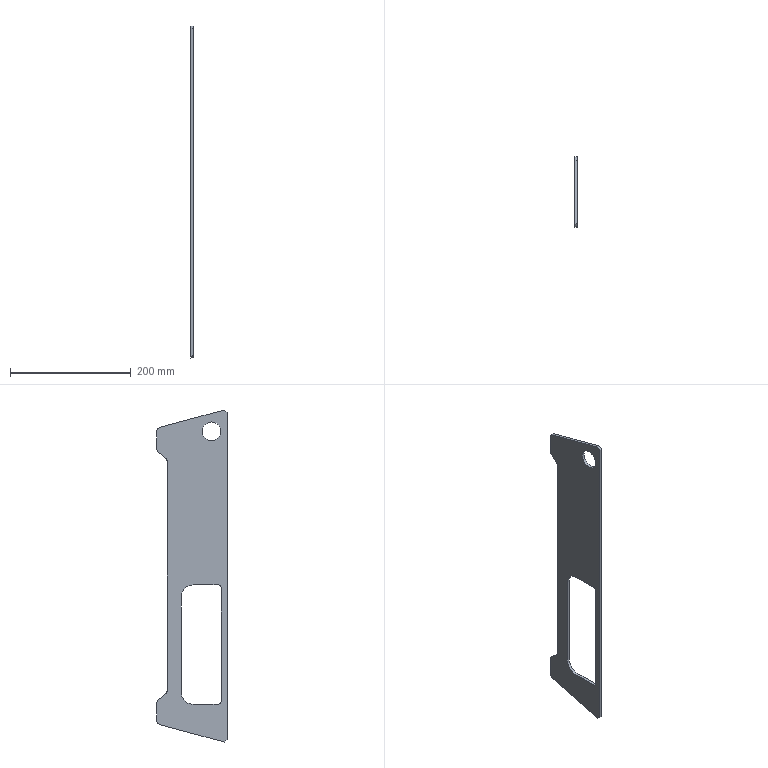Part | SolidWorks | features BaseBody 1 | 1 solid | 28 faces | box 4.5 x 116.8 x 550.797 mm | volume 181763 mm3 | plane 16 | cylinder 12 | commonest cylinder face diameters 16 x4 10 x2 12 x2 31 x2 40 x2
STEP:
#1=CARTESIAN_POINT('',(1093.2,55.3,688.5));
#2=VERTEX_POINT('',#1);
#3=CARTESIAN_POINT('',(1093.2,55.3,719.5));
#4=VERTEX_POINT('',#3);
#5=CARTESIAN_POINT('',(1093.2,55.3,704.));
#6=DIRECTION('',(-1.,0.,0.));
#7=DIRECTION('',(0.,0.,-1.));
#8=AXIS2_PLACEMENT_3D('',#5,#6,#7);
#9=CIRCLE('',#8,15.5);
#10=EDGE_CURVE('',#2,#4,#9,.T.);
#11=ORIENTED_EDGE('',*,*,#10,.T.);
#12=CARTESIAN_POINT('',(1097.7,55.3,719.5));
#13=VERTEX_POINT('',#12);
#14=CARTESIAN_POINT('',(1093.2,55.3,719.5));
#15=DIRECTION('',(1.,0.,0.));
#16=VECTOR('',#15,1000.);
#17=LINE('',#14,#16);
#18=EDGE_CURVE('',#4,#13,#17,.T.);
#19=ORIENTED_EDGE('',*,*,#18,.T.);
#20=CARTESIAN_POINT('',(1097.7,55.3,688.5));
#21=VERTEX_POINT('',#20);
#22=CARTESIAN_POINT('',(1097.7,55.3,704.));
#23=DIRECTION('',(-1.,0.,0.));
#24=DIRECTION('',(0.,0.,-1.));
#25=AXIS2_PLACEMENT_3D('',#22,#23,#24);
#26=CIRCLE('',#25,15.5);
#27=EDGE_CURVE('',#21,#13,#26,.T.);
#28=ORIENTED_EDGE('',*,*,#27,.F.);
#29=CARTESIAN_POINT('',(1093.2,55.3,688.5));
#30=DIRECTION('',(1.,0.,0.));
#31=VECTOR('',#30,1000.);
#32=LINE('',#29,#31);
#33=EDGE_CURVE('',#2,#21,#32,.T.);
#34=ORIENTED_EDGE('',*,*,#33,.F.);
#35=EDGE_LOOP('',(#11,#19,#28,#34));
#36=FACE_OUTER_BOUND('',#35,.T.);
#37=CARTESIAN_POINT('',(1093.2,55.3,704.));
#38=DIRECTION('',(1.,0.,0.));
#39=DIRECTION('',(0.,0.,-1.));
#40=AXIS2_PLACEMENT_3D('',#37,#38,#39);
#41=CYLINDRICAL_SURFACE('',#40,15.5);
#42=ADVANCED_FACE('',(#36),#41,.F.);
#43=CARTESIAN_POINT('',(1097.7,39.3,444.2));
#44=VERTEX_POINT('',#43);
#45=CARTESIAN_POINT('',(1097.7,44.3,449.2));
#46=VERTEX_POINT('',#45);
#47=CARTESIAN_POINT('',(1097.7,44.3,444.2));
#48=DIRECTION('',(-1.,0.,0.));
#49=DIRECTION('',(0.,0.,1.));
#50=AXIS2_PLACEMENT_3D('',#47,#48,#49);
#51=CIRCLE('',#50,5.);
#52=EDGE_CURVE('',#44,#46,#51,.T.);
#53=ORIENTED_EDGE('',*,*,#52,.T.);
#54=CARTESIAN_POINT('',(1097.7,85.7,449.2));
#55=VERTEX_POINT('',#54);
#56=CARTESIAN_POINT('',(1097.7,87.7,449.2));
#57=DIRECTION('',(0.,1.,0.));
#58=VECTOR('',#57,1000.);
#59=LINE('',#56,#58);
#60=EDGE_CURVE('',#46,#55,#59,.T.);
#61=ORIENTED_EDGE('',*,*,#60,.T.);
#62=CARTESIAN_POINT('',(1097.7,105.7,429.2));
#63=VERTEX_POINT('',#62);
#64=CARTESIAN_POINT('',(1097.7,85.7,429.2));
#65=DIRECTION('',(-1.,0.,0.));
#66=DIRECTION('',(0.,0.,1.));
#67=AXIS2_PLACEMENT_3D('',#64,#65,#66);
#68=CIRCLE('',#67,20.);
#69=EDGE_CURVE('',#55,#63,#68,.T.);
#70=ORIENTED_EDGE('',*,*,#69,.T.);
#71=CARTESIAN_POINT('',(1097.7,105.7,271.2));
#72=VERTEX_POINT('',#71);
#73=CARTESIAN_POINT('',(1097.7,105.7,464.));
#74=DIRECTION('',(0.,0.,-1.));
#75=VECTOR('',#74,1000.);
#76=LINE('',#73,#75);
#77=EDGE_CURVE('',#63,#72,#76,.T.);
#78=ORIENTED_EDGE('',*,*,#77,.T.);
#79=CARTESIAN_POINT('',(1097.7,85.7,251.2));
#80=VERTEX_POINT('',#79);
#81=CARTESIAN_POINT('',(1097.7,85.7,271.2));
#82=DIRECTION('',(-1.,0.,0.));
#83=DIRECTION('',(0.,0.,1.));
#84=AXIS2_PLACEMENT_3D('',#81,#82,#83);
#85=CIRCLE('',#84,20.);
#86=EDGE_CURVE('',#72,#80,#85,.T.);
#87=ORIENTED_EDGE('',*,*,#86,.T.);
#88=CARTESIAN_POINT('',(1097.7,44.3,251.2));
#89=VERTEX_POINT('',#88);
#90=CARTESIAN_POINT('',(1097.7,87.7,251.2));
#91=DIRECTION('',(0.,-1.,0.));
#92=VECTOR('',#91,1000.);
#93=LINE('',#90,#92);
#94=EDGE_CURVE('',#80,#89,#93,.T.);
#95=ORIENTED_EDGE('',*,*,#94,.T.);
#96=CARTESIAN_POINT('',(1097.7,39.3,256.2));
#97=VERTEX_POINT('',#96);
#98=CARTESIAN_POINT('',(1097.7,44.3,256.2));
#99=DIRECTION('',(-1.,0.,0.));
#100=DIRECTION('',(0.,0.,1.));
#101=AXIS2_PLACEMENT_3D('',#98,#99,#100);
#102=CIRCLE('',#101,5.);
#103=EDGE_CURVE('',#89,#97,#102,.T.);
#104=ORIENTED_EDGE('',*,*,#103,.T.);
#105=CARTESIAN_POINT('',(1097.7,39.3,464.));
#106=DIRECTION('',(0.,0.,1.));
#107=VECTOR('',#106,1000.);
#108=LINE('',#105,#107);
#109=EDGE_CURVE('',#97,#44,#108,.T.);
#110=ORIENTED_EDGE('',*,*,#109,.T.);
#111=EDGE_LOOP('',(#53,#61,#70,#78,#87,#95,#104,#110));
#112=FACE_BOUND('',#111,.T.);
#113=ORIENTED_EDGE('',*,*,#27,.T.);
#114=CARTESIAN_POINT('',(1097.7,55.3,704.));
#115=DIRECTION('',(-1.,0.,0.));
#116=DIRECTION('',(0.,0.,-1.));
#117=AXIS2_PLACEMENT_3D('',#114,#115,#116);
#118=CIRCLE('',#117,15.5);
#119=EDGE_CURVE('',#13,#21,#118,.T.);
#120=ORIENTED_EDGE('',*,*,#119,.T.);
#121=EDGE_LOOP('',(#113,#120));
#122=FACE_BOUND('',#121,.T.);
#123=CARTESIAN_POINT('',(1097.7,29.3,735.693));
#124=VERTEX_POINT('',#123);
#125=CARTESIAN_POINT('',(1097.7,29.3,192.307));
#126=VERTEX_POINT('',#125);
#127=CARTESIAN_POINT('',(1097.7,29.3,464.));
#128=DIRECTION('',(0.,0.,-1.));
#129=VECTOR('',#128,1000.);
#130=LINE('',#127,#129);
#131=EDGE_CURVE('',#124,#126,#130,.T.);
#132=ORIENTED_EDGE('',*,*,#131,.T.);
#133=CARTESIAN_POINT('',(1097.7,34.13,188.602));
#134=VERTEX_POINT('',#133);
#135=CARTESIAN_POINT('',(1097.7,29.3,192.307));
#136=DIRECTION('',(0.,0.7934,-0.6088));
#137=VECTOR('',#136,1000.);
#138=LINE('',#135,#137);
#139=EDGE_CURVE('',#126,#134,#138,.T.);
#140=ORIENTED_EDGE('',*,*,#139,.T.);
#141=CARTESIAN_POINT('',(1097.7,140.171,217.015));
#142=VERTEX_POINT('',#141);
#143=CARTESIAN_POINT('',(1097.7,34.13,188.602));
#144=DIRECTION('',(0.,0.9659,0.2588));
#145=VECTOR('',#144,1000.);
#146=LINE('',#143,#145);
#147=EDGE_CURVE('',#134,#142,#146,.T.);
#148=ORIENTED_EDGE('',*,*,#147,.T.);
#149=CARTESIAN_POINT('',(1097.7,146.1,224.743));
#150=VERTEX_POINT('',#149);
#151=CARTESIAN_POINT('',(1097.7,138.1,224.743));
#152=DIRECTION('',(1.,0.,0.));
#153=DIRECTION('',(0.,0.,1.));
#154=AXIS2_PLACEMENT_3D('',#151,#152,#153);
#155=CIRCLE('',#154,8.);
#156=EDGE_CURVE('',#142,#150,#155,.T.);
#157=ORIENTED_EDGE('',*,*,#156,.T.);
#158=CARTESIAN_POINT('',(1097.7,146.1,252.393));
#159=VERTEX_POINT('',#158);
#160=CARTESIAN_POINT('',(1097.7,146.1,464.));
#161=DIRECTION('',(0.,0.,1.));
#162=VECTOR('',#161,1000.);
#163=LINE('',#160,#162);
#164=EDGE_CURVE('',#150,#159,#163,.T.);
#165=ORIENTED_EDGE('',*,*,#164,.T.);
#166=CARTESIAN_POINT('',(1097.7,143.186,258.568));
#167=VERTEX_POINT('',#166);
#168=CARTESIAN_POINT('',(1097.7,138.1,252.393));
#169=DIRECTION('',(1.,0.,0.));
#170=DIRECTION('',(0.,0.,1.));
#171=AXIS2_PLACEMENT_3D('',#168,#169,#170);
#172=CIRCLE('',#171,8.);
#173=EDGE_CURVE('',#159,#167,#172,.T.);
#174=ORIENTED_EDGE('',*,*,#173,.T.);
#175=CARTESIAN_POINT('',(1097.7,131.286,268.368));
#176=VERTEX_POINT('',#175);
#177=CARTESIAN_POINT('',(1097.7,143.186,258.568));
#178=DIRECTION('',(0.,-0.7719,0.6357));
#179=VECTOR('',#178,1000.);
#180=LINE('',#177,#179);
#181=EDGE_CURVE('',#167,#176,#180,.T.);
#182=ORIENTED_EDGE('',*,*,#181,.T.);
#183=CARTESIAN_POINT('',(1097.7,129.1,273.));
#184=VERTEX_POINT('',#183);
#185=CARTESIAN_POINT('',(1097.7,135.1,273.));
#186=DIRECTION('',(-1.,0.,0.));
#187=DIRECTION('',(0.,0.,-1.));
#188=AXIS2_PLACEMENT_3D('',#185,#186,#187);
#189=CIRCLE('',#188,6.);
#190=EDGE_CURVE('',#176,#184,#189,.T.);
#191=ORIENTED_EDGE('',*,*,#190,.T.);
#192=CARTESIAN_POINT('',(1097.7,129.1,655.));
#193=VERTEX_POINT('',#192);
#194=CARTESIAN_POINT('',(1097.7,129.1,464.));
#195=DIRECTION('',(0.,0.,1.));
#196=VECTOR('',#195,1000.);
#197=LINE('',#194,#196);
#198=EDGE_CURVE('',#184,#193,#197,.T.);
#199=ORIENTED_EDGE('',*,*,#198,.T.);
#200=CARTESIAN_POINT('',(1097.7,131.286,659.632));
#201=VERTEX_POINT('',#200);
#202=CARTESIAN_POINT('',(1097.7,135.1,655.));
#203=DIRECTION('',(-1.,0.,0.));
#204=DIRECTION('',(0.,0.,-1.));
#205=AXIS2_PLACEMENT_3D('',#202,#203,#204);
#206=CIRCLE('',#205,6.);
#207=EDGE_CURVE('',#193,#201,#206,.T.);
#208=ORIENTED_EDGE('',*,*,#207,.T.);
#209=CARTESIAN_POINT('',(1097.7,143.186,669.432));
#210=VERTEX_POINT('',#209);
#211=CARTESIAN_POINT('',(1097.7,131.286,659.632));
#212=DIRECTION('',(0.,0.7719,0.6357));
#213=VECTOR('',#212,1000.);
#214=LINE('',#211,#213);
#215=EDGE_CURVE('',#201,#210,#214,.T.);
#216=ORIENTED_EDGE('',*,*,#215,.T.);
#217=CARTESIAN_POINT('',(1097.7,146.1,675.607));
#218=VERTEX_POINT('',#217);
#219=CARTESIAN_POINT('',(1097.7,138.1,675.607));
#220=DIRECTION('',(1.,0.,0.));
#221=DIRECTION('',(0.,0.,1.));
#222=AXIS2_PLACEMENT_3D('',#219,#220,#221);
#223=CIRCLE('',#222,8.);
#224=EDGE_CURVE('',#210,#218,#223,.T.);
#225=ORIENTED_EDGE('',*,*,#224,.T.);
#226=CARTESIAN_POINT('',(1097.7,146.1,703.257));
#227=VERTEX_POINT('',#226);
#228=CARTESIAN_POINT('',(1097.7,146.1,464.));
#229=DIRECTION('',(0.,0.,1.));
#230=VECTOR('',#229,1000.);
#231=LINE('',#228,#230);
#232=EDGE_CURVE('',#218,#227,#231,.T.);
#233=ORIENTED_EDGE('',*,*,#232,.T.);
#234=CARTESIAN_POINT('',(1097.7,140.171,710.985));
#235=VERTEX_POINT('',#234);
#236=CARTESIAN_POINT('',(1097.7,138.1,703.257));
#237=DIRECTION('',(1.,0.,0.));
#238=DIRECTION('',(0.,0.,1.));
#239=AXIS2_PLACEMENT_3D('',#236,#237,#238);
#240=CIRCLE('',#239,8.);
#241=EDGE_CURVE('',#227,#235,#240,.T.);
#242=ORIENTED_EDGE('',*,*,#241,.T.);
#243=CARTESIAN_POINT('',(1097.7,34.13,739.398));
#244=VERTEX_POINT('',#243);
#245=CARTESIAN_POINT('',(1097.7,140.171,710.985));
#246=DIRECTION('',(0.,-0.9659,0.2588));
#247=VECTOR('',#246,1000.);
#248=LINE('',#245,#247);
#249=EDGE_CURVE('',#235,#244,#248,.T.);
#250=ORIENTED_EDGE('',*,*,#249,.T.);
#251=CARTESIAN_POINT('',(1097.7,34.13,739.398));
#252=DIRECTION('',(0.,-0.7934,-0.6088));
#253=VECTOR('',#252,1000.);
#254=LINE('',#251,#253);
#255=EDGE_CURVE('',#244,#124,#254,.T.);
#256=ORIENTED_EDGE('',*,*,#255,.T.);
#257=EDGE_LOOP('',(#132,#140,#148,#157,#165,#174,#182,#191,#199,#208,#216,#225,#233,#242,#250,#256));
#258=FACE_OUTER_BOUND('',#257,.T.);
#259=CARTESIAN_POINT('',(1097.7,29.3,185.297));
#260=DIRECTION('',(1.,0.,0.));
#261=DIRECTION('',(0.,1.,0.));
#262=AXIS2_PLACEMENT_3D('',#259,#260,#261);
#263=PLANE('',#262);
#264=ADVANCED_FACE('',(#112,#122,#258),#263,.T.);
#265=CARTESIAN_POINT('',(1093.2,85.7,449.2));
#266=VERTEX_POINT('',#265);
#267=CARTESIAN_POINT('',(1095.45,85.7,449.2));
#268=DIRECTION('',(-1.,0.,0.));
#269=VECTOR('',#268,1000.);
#270=LINE('',#267,#269);
#271=EDGE_CURVE('',#55,#266,#270,.T.);
#272=ORIENTED_EDGE('',*,*,#271,.F.);
#273=ORIENTED_EDGE('',*,*,#60,.F.);
#274=CARTESIAN_POINT('',(1093.2,44.3,449.2));
#275=VERTEX_POINT('',#274);
#276=CARTESIAN_POINT('',(1095.45,44.3,449.2));
#277=DIRECTION('',(1.,0.,0.));
#278=VECTOR('',#277,1000.);
#279=LINE('',#276,#278);
#280=EDGE_CURVE('',#275,#46,#279,.T.);
#281=ORIENTED_EDGE('',*,*,#280,.F.);
#282=CARTESIAN_POINT('',(1093.2,65.,449.2));
#283=DIRECTION('',(0.,-1.,0.));
#284=VECTOR('',#283,1000.);
#285=LINE('',#282,#284);
#286=EDGE_CURVE('',#266,#275,#285,.T.);
#287=ORIENTED_EDGE('',*,*,#286,.F.);
#288=EDGE_LOOP('',(#272,#273,#281,#287));
#289=FACE_OUTER_BOUND('',#288,.T.);
#290=CARTESIAN_POINT('',(1093.2,44.3,449.2));
#291=DIRECTION('',(0.,0.,1.));
#292=DIRECTION('',(1.,0.,0.));
#293=AXIS2_PLACEMENT_3D('',#290,#291,#292);
#294=PLANE('',#293);
#295=ADVANCED_FACE('',(#289),#294,.F.);
#296=ORIENTED_EDGE('',*,*,#52,.F.);
#297=CARTESIAN_POINT('',(1093.2,39.3,444.2));
#298=VERTEX_POINT('',#297);
#299=CARTESIAN_POINT('',(1095.45,39.3,444.2));
#300=DIRECTION('',(-1.,0.,0.));
#301=VECTOR('',#300,1000.);
#302=LINE('',#299,#301);
#303=EDGE_CURVE('',#44,#298,#302,.T.);
#304=ORIENTED_EDGE('',*,*,#303,.T.);
#305=CARTESIAN_POINT('',(1093.2,44.3,444.2));
#306=DIRECTION('',(-1.,0.,0.));
#307=DIRECTION('',(0.,0.,1.));
#308=AXIS2_PLACEMENT_3D('',#305,#306,#307);
#309=CIRCLE('',#308,5.);
#310=EDGE_CURVE('',#298,#275,#309,.T.);
#311=ORIENTED_EDGE('',*,*,#310,.T.);
#312=ORIENTED_EDGE('',*,*,#280,.T.);
#313=EDGE_LOOP('',(#296,#304,#311,#312));
#314=FACE_OUTER_BOUND('',#313,.T.);
#315=CARTESIAN_POINT('',(1097.7,44.3,444.2));
#316=DIRECTION('',(-1.,0.,0.));
#317=DIRECTION('',(0.,0.,1.));
#318=AXIS2_PLACEMENT_3D('',#315,#316,#317);
#319=CYLINDRICAL_SURFACE('',#318,5.);
#320=ADVANCED_FACE('',(#314),#319,.F.);
#321=ORIENTED_EDGE('',*,*,#303,.F.);
#322=ORIENTED_EDGE('',*,*,#109,.F.);
#323=CARTESIAN_POINT('',(1093.2,39.3,256.2));
#324=VERTEX_POINT('',#323);
#325=CARTESIAN_POINT('',(1095.45,39.3,256.2));
#326=DIRECTION('',(1.,0.,0.));
#327=VECTOR('',#326,1000.);
#328=LINE('',#325,#327);
#329=EDGE_CURVE('',#324,#97,#328,.T.);
#330=ORIENTED_EDGE('',*,*,#329,.F.);
#331=CARTESIAN_POINT('',(1093.2,39.3,350.2));
#332=DIRECTION('',(0.,0.,-1.));
#333=VECTOR('',#332,1000.);
#334=LINE('',#331,#333);
#335=EDGE_CURVE('',#298,#324,#334,.T.);
#336=ORIENTED_EDGE('',*,*,#335,.F.);
#337=EDGE_LOOP('',(#321,#322,#330,#336));
#338=FACE_OUTER_BOUND('',#337,.T.);
#339=CARTESIAN_POINT('',(1093.2,39.3,444.2));
#340=DIRECTION('',(0.,-1.,0.));
#341=DIRECTION('',(0.,0.,-1.));
#342=AXIS2_PLACEMENT_3D('',#339,#340,#341);
#343=PLANE('',#342);
#344=ADVANCED_FACE('',(#338),#343,.F.);
#345=ORIENTED_EDGE('',*,*,#103,.F.);
#346=CARTESIAN_POINT('',(1093.2,44.3,251.2));
#347=VERTEX_POINT('',#346);
#348=CARTESIAN_POINT('',(1095.45,44.3,251.2));
#349=DIRECTION('',(-1.,0.,0.));
#350=VECTOR('',#349,1000.);
#351=LINE('',#348,#350);
#352=EDGE_CURVE('',#89,#347,#351,.T.);
#353=ORIENTED_EDGE('',*,*,#352,.T.);
#354=CARTESIAN_POINT('',(1093.2,44.3,256.2));
#355=DIRECTION('',(-1.,0.,0.));
#356=DIRECTION('',(0.,0.,1.));
#357=AXIS2_PLACEMENT_3D('',#354,#355,#356);
#358=CIRCLE('',#357,5.);
#359=EDGE_CURVE('',#347,#324,#358,.T.);
#360=ORIENTED_EDGE('',*,*,#359,.T.);
#361=ORIENTED_EDGE('',*,*,#329,.T.);
#362=EDGE_LOOP('',(#345,#353,#360,#361));
#363=FACE_OUTER_BOUND('',#362,.T.);
#364=CARTESIAN_POINT('',(1097.7,44.3,256.2));
#365=DIRECTION('',(-1.,0.,0.));
#366=DIRECTION('',(0.,0.,1.));
#367=AXIS2_PLACEMENT_3D('',#364,#365,#366);
#368=CYLINDRICAL_SURFACE('',#367,5.);
#369=ADVANCED_FACE('',(#363),#368,.F.);
#370=CARTESIAN_POINT('',(1093.2,85.7,251.2));
#371=VERTEX_POINT('',#370);
#372=CARTESIAN_POINT('',(1095.45,85.7,251.2));
#373=DIRECTION('',(1.,0.,0.));
#374=VECTOR('',#373,1000.);
#375=LINE('',#372,#374);
#376=EDGE_CURVE('',#371,#80,#375,.T.);
#377=ORIENTED_EDGE('',*,*,#376,.F.);
#378=CARTESIAN_POINT('',(1093.2,65.,251.2));
#379=DIRECTION('',(0.,1.,0.));
#380=VECTOR('',#379,1000.);
#381=LINE('',#378,#380);
#382=EDGE_CURVE('',#347,#371,#381,.T.);
#383=ORIENTED_EDGE('',*,*,#382,.F.);
#384=ORIENTED_EDGE('',*,*,#352,.F.);
#385=ORIENTED_EDGE('',*,*,#94,.F.);
#386=EDGE_LOOP('',(#377,#383,#384,#385));
#387=FACE_OUTER_BOUND('',#386,.T.);
#388=CARTESIAN_POINT('',(1097.7,85.7,251.2));
#389=DIRECTION('',(0.,0.,-1.));
#390=DIRECTION('',(0.,-1.,0.));
#391=AXIS2_PLACEMENT_3D('',#388,#389,#390);
#392=PLANE('',#391);
#393=ADVANCED_FACE('',(#387),#392,.F.);
#394=ORIENTED_EDGE('',*,*,#86,.F.);
#395=CARTESIAN_POINT('',(1093.2,105.7,271.2));
#396=VERTEX_POINT('',#395);
#397=CARTESIAN_POINT('',(1095.45,105.7,271.2));
#398=DIRECTION('',(-1.,0.,0.));
#399=VECTOR('',#398,1000.);
#400=LINE('',#397,#399);
#401=EDGE_CURVE('',#72,#396,#400,.T.);
#402=ORIENTED_EDGE('',*,*,#401,.T.);
#403=CARTESIAN_POINT('',(1093.2,85.7,271.2));
#404=DIRECTION('',(-1.,0.,0.));
#405=DIRECTION('',(0.,0.,1.));
#406=AXIS2_PLACEMENT_3D('',#403,#404,#405);
#407=CIRCLE('',#406,20.);
#408=EDGE_CURVE('',#396,#371,#407,.T.);
#409=ORIENTED_EDGE('',*,*,#408,.T.);
#410=ORIENTED_EDGE('',*,*,#376,.T.);
#411=EDGE_LOOP('',(#394,#402,#409,#410));
#412=FACE_OUTER_BOUND('',#411,.T.);
#413=CARTESIAN_POINT('',(1097.7,85.7,271.2));
#414=DIRECTION('',(-1.,0.,0.));
#415=DIRECTION('',(0.,0.,1.));
#416=AXIS2_PLACEMENT_3D('',#413,#414,#415);
#417=CYLINDRICAL_SURFACE('',#416,20.);
#418=ADVANCED_FACE('',(#412),#417,.F.);
#419=CARTESIAN_POINT('',(1093.2,105.7,429.2));
#420=VERTEX_POINT('',#419);
#421=CARTESIAN_POINT('',(1095.45,105.7,429.2));
#422=DIRECTION('',(1.,0.,0.));
#423=VECTOR('',#422,1000.);
#424=LINE('',#421,#423);
#425=EDGE_CURVE('',#420,#63,#424,.T.);
#426=ORIENTED_EDGE('',*,*,#425,.F.);
#427=CARTESIAN_POINT('',(1093.2,105.7,350.2));
#428=DIRECTION('',(0.,0.,1.));
#429=VECTOR('',#428,1000.);
#430=LINE('',#427,#429);
#431=EDGE_CURVE('',#396,#420,#430,.T.);
#432=ORIENTED_EDGE('',*,*,#431,.F.);
#433=ORIENTED_EDGE('',*,*,#401,.F.);
#434=ORIENTED_EDGE('',*,*,#77,.F.);
#435=EDGE_LOOP('',(#426,#432,#433,#434));
#436=FACE_OUTER_BOUND('',#435,.T.);
#437=CARTESIAN_POINT('',(1093.2,105.7,429.2));
#438=DIRECTION('',(0.,1.,0.));
#439=DIRECTION('',(1.,0.,0.));
#440=AXIS2_PLACEMENT_3D('',#437,#438,#439);
#441=PLANE('',#440);
#442=ADVANCED_FACE('',(#436),#441,.F.);
#443=ORIENTED_EDGE('',*,*,#69,.F.);
#444=ORIENTED_EDGE('',*,*,#271,.T.);
#445=CARTESIAN_POINT('',(1093.2,85.7,429.2));
#446=DIRECTION('',(-1.,0.,0.));
#447=DIRECTION('',(0.,0.,1.));
#448=AXIS2_PLACEMENT_3D('',#445,#446,#447);
#449=CIRCLE('',#448,20.);
#450=EDGE_CURVE('',#266,#420,#449,.T.);
#451=ORIENTED_EDGE('',*,*,#450,.T.);
#452=ORIENTED_EDGE('',*,*,#425,.T.);
#453=EDGE_LOOP('',(#443,#444,#451,#452));
#454=FACE_OUTER_BOUND('',#453,.T.);
#455=CARTESIAN_POINT('',(1097.7,85.7,429.2));
#456=DIRECTION('',(-1.,0.,0.));
#457=DIRECTION('',(0.,0.,1.));
#458=AXIS2_PLACEMENT_3D('',#455,#456,#457);
#459=CYLINDRICAL_SURFACE('',#458,20.);
#460=ADVANCED_FACE('',(#454),#459,.F.);
#461=ORIENTED_EDGE('',*,*,#18,.F.);
#462=CARTESIAN_POINT('',(1093.2,55.3,704.));
#463=DIRECTION('',(-1.,0.,0.));
#464=DIRECTION('',(0.,0.,-1.));
#465=AXIS2_PLACEMENT_3D('',#462,#463,#464);
#466=CIRCLE('',#465,15.5);
#467=EDGE_CURVE('',#4,#2,#466,.T.);
#468=ORIENTED_EDGE('',*,*,#467,.T.);
#469=ORIENTED_EDGE('',*,*,#33,.T.);
#470=ORIENTED_EDGE('',*,*,#119,.F.);
#471=EDGE_LOOP('',(#461,#468,#469,#470));
#472=FACE_OUTER_BOUND('',#471,.T.);
#473=CARTESIAN_POINT('',(1093.2,55.3,704.));
#474=DIRECTION('',(1.,0.,0.));
#475=DIRECTION('',(0.,0.,-1.));
#476=AXIS2_PLACEMENT_3D('',#473,#474,#475);
#477=CYLINDRICAL_SURFACE('',#476,15.5);
#478=ADVANCED_FACE('',(#472),#477,.F.);
#479=CARTESIAN_POINT('',(1093.2,29.3,192.307));
#480=VERTEX_POINT('',#479);
#481=CARTESIAN_POINT('',(1095.45,29.3,192.307));
#482=DIRECTION('',(-1.,0.,0.));
#483=VECTOR('',#482,1000.);
#484=LINE('',#481,#483);
#485=EDGE_CURVE('',#126,#480,#484,.T.);
#486=ORIENTED_EDGE('',*,*,#485,.T.);
#487=CARTESIAN_POINT('',(1093.2,34.13,188.602));
#488=VERTEX_POINT('',#487);
#489=CARTESIAN_POINT('',(1093.2,31.715,190.455));
#490=DIRECTION('',(0.,0.7934,-0.6088));
#491=VECTOR('',#490,1000.);
#492=LINE('',#489,#491);
#493=EDGE_CURVE('',#480,#488,#492,.T.);
#494=ORIENTED_EDGE('',*,*,#493,.T.);
#495=CARTESIAN_POINT('',(1095.45,34.13,188.602));
#496=DIRECTION('',(1.,0.,0.));
#497=VECTOR('',#496,1000.);
#498=LINE('',#495,#497);
#499=EDGE_CURVE('',#488,#134,#498,.T.);
#500=ORIENTED_EDGE('',*,*,#499,.T.);
#501=ORIENTED_EDGE('',*,*,#139,.F.);
#502=EDGE_LOOP('',(#486,#494,#500,#501));
#503=FACE_OUTER_BOUND('',#502,.T.);
#504=CARTESIAN_POINT('',(1097.7,34.13,188.602));
#505=DIRECTION('',(0.,-0.6088,-0.7934));
#506=DIRECTION('',(0.,-0.7934,0.6088));
#507=AXIS2_PLACEMENT_3D('',#504,#505,#506);
#508=PLANE('',#507);
#509=ADVANCED_FACE('',(#503),#508,.T.);
#510=CARTESIAN_POINT('',(1093.2,29.3,735.693));
#511=VERTEX_POINT('',#510);
#512=CARTESIAN_POINT('',(1093.2,29.3,464.));
#513=DIRECTION('',(0.,0.,-1.));
#514=VECTOR('',#513,1000.);
#515=LINE('',#512,#514);
#516=EDGE_CURVE('',#511,#480,#515,.T.);
#517=ORIENTED_EDGE('',*,*,#516,.T.);
#518=ORIENTED_EDGE('',*,*,#485,.F.);
#519=ORIENTED_EDGE('',*,*,#131,.F.);
#520=CARTESIAN_POINT('',(1095.45,29.3,735.693));
#521=DIRECTION('',(-1.,0.,0.));
#522=VECTOR('',#521,1000.);
#523=LINE('',#520,#522);
#524=EDGE_CURVE('',#124,#511,#523,.T.);
#525=ORIENTED_EDGE('',*,*,#524,.T.);
#526=EDGE_LOOP('',(#517,#518,#519,#525));
#527=FACE_OUTER_BOUND('',#526,.T.);
#528=CARTESIAN_POINT('',(1093.2,29.3,735.693));
#529=DIRECTION('',(0.,-1.,0.));
#530=DIRECTION('',(0.,0.,-1.));
#531=AXIS2_PLACEMENT_3D('',#528,#529,#530);
#532=PLANE('',#531);
#533=ADVANCED_FACE('',(#527),#532,.T.);
#534=CARTESIAN_POINT('',(1093.2,34.13,739.398));
#535=VERTEX_POINT('',#534);
#536=CARTESIAN_POINT('',(1095.45,34.13,739.398));
#537=DIRECTION('',(-1.,0.,0.));
#538=VECTOR('',#537,1000.);
#539=LINE('',#536,#538);
#540=EDGE_CURVE('',#244,#535,#539,.T.);
#541=ORIENTED_EDGE('',*,*,#540,.T.);
#542=CARTESIAN_POINT('',(1093.2,31.715,737.545));
#543=DIRECTION('',(0.,-0.7934,-0.6088));
#544=VECTOR('',#543,1000.);
#545=LINE('',#542,#544);
#546=EDGE_CURVE('',#535,#511,#545,.T.);
#547=ORIENTED_EDGE('',*,*,#546,.T.);
#548=ORIENTED_EDGE('',*,*,#524,.F.);
#549=ORIENTED_EDGE('',*,*,#255,.F.);
#550=EDGE_LOOP('',(#541,#547,#548,#549));
#551=FACE_OUTER_BOUND('',#550,.T.);
#552=CARTESIAN_POINT('',(1097.7,34.13,739.398));
#553=DIRECTION('',(0.,-0.6088,0.7934));
#554=DIRECTION('',(-1.,0.,0.));
#555=AXIS2_PLACEMENT_3D('',#552,#553,#554);
#556=PLANE('',#555);
#557=ADVANCED_FACE('',(#551),#556,.T.);
#558=CARTESIAN_POINT('',(1093.2,140.171,710.985));
#559=VERTEX_POINT('',#558);
#560=CARTESIAN_POINT('',(1093.2,87.15,725.192));
#561=DIRECTION('',(0.,-0.9659,0.2588));
#562=VECTOR('',#561,1000.);
#563=LINE('',#560,#562);
#564=EDGE_CURVE('',#559,#535,#563,.T.);
#565=ORIENTED_EDGE('',*,*,#564,.T.);
#566=ORIENTED_EDGE('',*,*,#540,.F.);
#567=ORIENTED_EDGE('',*,*,#249,.F.);
#568=CARTESIAN_POINT('',(1095.45,140.171,710.985));
#569=DIRECTION('',(-1.,0.,0.));
#570=VECTOR('',#569,1000.);
#571=LINE('',#568,#570);
#572=EDGE_CURVE('',#235,#559,#571,.T.);
#573=ORIENTED_EDGE('',*,*,#572,.T.);
#574=EDGE_LOOP('',(#565,#566,#567,#573));
#575=FACE_OUTER_BOUND('',#574,.T.);
#576=CARTESIAN_POINT('',(1093.2,34.13,739.398));
#577=DIRECTION('',(0.,0.2588,0.9659));
#578=DIRECTION('',(1.,0.,0.));
#579=AXIS2_PLACEMENT_3D('',#576,#577,#578);
#580=PLANE('',#579);
#581=ADVANCED_FACE('',(#575),#580,.T.);
#582=ORIENTED_EDGE('',*,*,#241,.F.);
#583=CARTESIAN_POINT('',(1093.2,146.1,703.257));
#584=VERTEX_POINT('',#583);
#585=CARTESIAN_POINT('',(1095.45,146.1,703.257));
#586=DIRECTION('',(1.,0.,0.));
#587=VECTOR('',#586,1000.);
#588=LINE('',#585,#587);
#589=EDGE_CURVE('',#584,#227,#588,.T.);
#590=ORIENTED_EDGE('',*,*,#589,.F.);
#591=CARTESIAN_POINT('',(1093.2,138.1,703.257));
#592=DIRECTION('',(-1.,0.,0.));
#593=DIRECTION('',(0.,0.,1.));
#594=AXIS2_PLACEMENT_3D('',#591,#592,#593);
#595=CIRCLE('',#594,8.);
#596=EDGE_CURVE('',#559,#584,#595,.T.);
#597=ORIENTED_EDGE('',*,*,#596,.F.);
#598=ORIENTED_EDGE('',*,*,#572,.F.);
#599=EDGE_LOOP('',(#582,#590,#597,#598));
#600=FACE_OUTER_BOUND('',#599,.T.);
#601=CARTESIAN_POINT('',(1097.7,138.1,703.257));
#602=DIRECTION('',(-1.,0.,0.));
#603=DIRECTION('',(0.,0.,1.));
#604=AXIS2_PLACEMENT_3D('',#601,#602,#603);
#605=CYLINDRICAL_SURFACE('',#604,8.);
#606=ADVANCED_FACE('',(#600),#605,.T.);
#607=ORIENTED_EDGE('',*,*,#589,.T.);
#608=ORIENTED_EDGE('',*,*,#232,.F.);
#609=CARTESIAN_POINT('',(1093.2,146.1,675.607));
#610=VERTEX_POINT('',#609);
#611=CARTESIAN_POINT('',(1095.45,146.1,675.607));
#612=DIRECTION('',(-1.,0.,0.));
#613=VECTOR('',#612,1000.);
#614=LINE('',#611,#613);
#615=EDGE_CURVE('',#218,#610,#614,.T.);
#616=ORIENTED_EDGE('',*,*,#615,.T.);
#617=CARTESIAN_POINT('',(1093.2,146.1,689.432));
#618=DIRECTION('',(0.,0.,1.));
#619=VECTOR('',#618,1000.);
#620=LINE('',#617,#619);
#621=EDGE_CURVE('',#610,#584,#620,.T.);
#622=ORIENTED_EDGE('',*,*,#621,.T.);
#623=EDGE_LOOP('',(#607,#608,#616,#622));
#624=FACE_OUTER_BOUND('',#623,.T.);
#625=CARTESIAN_POINT('',(1093.2,146.1,703.257));
#626=DIRECTION('',(0.,1.,0.));
#627=DIRECTION('',(1.,0.,0.));
#628=AXIS2_PLACEMENT_3D('',#625,#626,#627);
#629=PLANE('',#628);
#630=ADVANCED_FACE('',(#624),#629,.T.);
#631=ORIENTED_EDGE('',*,*,#224,.F.);
#632=CARTESIAN_POINT('',(1093.2,143.186,669.432));
#633=VERTEX_POINT('',#632);
#634=CARTESIAN_POINT('',(1095.45,143.186,669.432));
#635=DIRECTION('',(1.,0.,0.));
#636=VECTOR('',#635,1000.);
#637=LINE('',#634,#636);
#638=EDGE_CURVE('',#633,#210,#637,.T.);
#639=ORIENTED_EDGE('',*,*,#638,.F.);
#640=CARTESIAN_POINT('',(1093.2,138.1,675.607));
#641=DIRECTION('',(-1.,0.,0.));
#642=DIRECTION('',(0.,0.,1.));
#643=AXIS2_PLACEMENT_3D('',#640,#641,#642);
#644=CIRCLE('',#643,8.);
#645=EDGE_CURVE('',#610,#633,#644,.T.);
#646=ORIENTED_EDGE('',*,*,#645,.F.);
#647=ORIENTED_EDGE('',*,*,#615,.F.);
#648=EDGE_LOOP('',(#631,#639,#646,#647));
#649=FACE_OUTER_BOUND('',#648,.T.);
#650=CARTESIAN_POINT('',(1097.7,138.1,675.607));
#651=DIRECTION('',(-1.,0.,0.));
#652=DIRECTION('',(0.,0.,1.));
#653=AXIS2_PLACEMENT_3D('',#650,#651,#652);
#654=CYLINDRICAL_SURFACE('',#653,8.);
#655=ADVANCED_FACE('',(#649),#654,.T.);
#656=CARTESIAN_POINT('',(1093.2,131.286,659.632));
#657=VERTEX_POINT('',#656);
#658=CARTESIAN_POINT('',(1093.2,137.236,664.532));
#659=DIRECTION('',(0.,0.7719,0.6357));
#660=VECTOR('',#659,1000.);
#661=LINE('',#658,#660);
#662=EDGE_CURVE('',#657,#633,#661,.T.);
#663=ORIENTED_EDGE('',*,*,#662,.T.);
#664=ORIENTED_EDGE('',*,*,#638,.T.);
#665=ORIENTED_EDGE('',*,*,#215,.F.);
#666=CARTESIAN_POINT('',(1095.45,131.286,659.632));
#667=DIRECTION('',(-1.,0.,0.));
#668=VECTOR('',#667,1000.);
#669=LINE('',#666,#668);
#670=EDGE_CURVE('',#201,#657,#669,.T.);
#671=ORIENTED_EDGE('',*,*,#670,.T.);
#672=EDGE_LOOP('',(#663,#664,#665,#671));
#673=FACE_OUTER_BOUND('',#672,.T.);
#674=CARTESIAN_POINT('',(1097.7,131.286,659.632));
#675=DIRECTION('',(0.,0.6357,-0.7719));
#676=DIRECTION('',(-1.,0.,0.));
#677=AXIS2_PLACEMENT_3D('',#674,#675,#676);
#678=PLANE('',#677);
#679=ADVANCED_FACE('',(#673),#678,.T.);
#680=CARTESIAN_POINT('',(1093.2,129.1,655.));
#681=VERTEX_POINT('',#680);
#682=CARTESIAN_POINT('',(1095.45,129.1,655.));
#683=DIRECTION('',(-1.,0.,0.));
#684=VECTOR('',#683,1000.);
#685=LINE('',#682,#684);
#686=EDGE_CURVE('',#193,#681,#685,.T.);
#687=ORIENTED_EDGE('',*,*,#686,.T.);
#688=CARTESIAN_POINT('',(1093.2,135.1,655.));
#689=DIRECTION('',(-1.,0.,0.));
#690=DIRECTION('',(0.,0.,-1.));
#691=AXIS2_PLACEMENT_3D('',#688,#689,#690);
#692=CIRCLE('',#691,6.);
#693=EDGE_CURVE('',#681,#657,#692,.T.);
#694=ORIENTED_EDGE('',*,*,#693,.T.);
#695=ORIENTED_EDGE('',*,*,#670,.F.);
#696=ORIENTED_EDGE('',*,*,#207,.F.);
#697=EDGE_LOOP('',(#687,#694,#695,#696));
#698=FACE_OUTER_BOUND('',#697,.T.);
#699=CARTESIAN_POINT('',(1093.2,135.1,655.));
#700=DIRECTION('',(1.,0.,0.));
#701=DIRECTION('',(0.,0.,-1.));
#702=AXIS2_PLACEMENT_3D('',#699,#700,#701);
#703=CYLINDRICAL_SURFACE('',#702,6.);
#704=ADVANCED_FACE('',(#698),#703,.F.);
#705=CARTESIAN_POINT('',(1093.2,129.1,273.));
#706=VERTEX_POINT('',#705);
#707=CARTESIAN_POINT('',(1093.2,129.1,464.));
#708=DIRECTION('',(0.,0.,1.));
#709=VECTOR('',#708,1000.);
#710=LINE('',#707,#709);
#711=EDGE_CURVE('',#706,#681,#710,.T.);
#712=ORIENTED_EDGE('',*,*,#711,.T.);
#713=ORIENTED_EDGE('',*,*,#686,.F.);
#714=ORIENTED_EDGE('',*,*,#198,.F.);
#715=CARTESIAN_POINT('',(1095.45,129.1,273.));
#716=DIRECTION('',(-1.,0.,0.));
#717=VECTOR('',#716,1000.);
#718=LINE('',#715,#717);
#719=EDGE_CURVE('',#184,#706,#718,.T.);
#720=ORIENTED_EDGE('',*,*,#719,.T.);
#721=EDGE_LOOP('',(#712,#713,#714,#720));
#722=FACE_OUTER_BOUND('',#721,.T.);
#723=CARTESIAN_POINT('',(1093.2,129.1,655.));
#724=DIRECTION('',(0.,1.,0.));
#725=DIRECTION('',(1.,0.,0.));
#726=AXIS2_PLACEMENT_3D('',#723,#724,#725);
#727=PLANE('',#726);
#728=ADVANCED_FACE('',(#722),#727,.T.);
#729=CARTESIAN_POINT('',(1093.2,131.286,268.368));
#730=VERTEX_POINT('',#729);
#731=CARTESIAN_POINT('',(1095.45,131.286,268.368));
#732=DIRECTION('',(-1.,0.,0.));
#733=VECTOR('',#732,1000.);
#734=LINE('',#731,#733);
#735=EDGE_CURVE('',#176,#730,#734,.T.);
#736=ORIENTED_EDGE('',*,*,#735,.T.);
#737=CARTESIAN_POINT('',(1093.2,135.1,273.));
#738=DIRECTION('',(-1.,0.,0.));
#739=DIRECTION('',(0.,0.,-1.));
#740=AXIS2_PLACEMENT_3D('',#737,#738,#739);
#741=CIRCLE('',#740,6.);
#742=EDGE_CURVE('',#730,#706,#741,.T.);
#743=ORIENTED_EDGE('',*,*,#742,.T.);
#744=ORIENTED_EDGE('',*,*,#719,.F.);
#745=ORIENTED_EDGE('',*,*,#190,.F.);
#746=EDGE_LOOP('',(#736,#743,#744,#745));
#747=FACE_OUTER_BOUND('',#746,.T.);
#748=CARTESIAN_POINT('',(1093.2,135.1,273.));
#749=DIRECTION('',(1.,0.,0.));
#750=DIRECTION('',(0.,0.,-1.));
#751=AXIS2_PLACEMENT_3D('',#748,#749,#750);
#752=CYLINDRICAL_SURFACE('',#751,6.);
#753=ADVANCED_FACE('',(#747),#752,.F.);
#754=ORIENTED_EDGE('',*,*,#181,.F.);
#755=CARTESIAN_POINT('',(1093.2,143.186,258.568));
#756=VERTEX_POINT('',#755);
#757=CARTESIAN_POINT('',(1095.45,143.186,258.568));
#758=DIRECTION('',(-1.,0.,0.));
#759=VECTOR('',#758,1000.);
#760=LINE('',#757,#759);
#761=EDGE_CURVE('',#167,#756,#760,.T.);
#762=ORIENTED_EDGE('',*,*,#761,.T.);
#763=CARTESIAN_POINT('',(1093.2,137.236,263.468));
#764=DIRECTION('',(0.,-0.7719,0.6357));
#765=VECTOR('',#764,1000.);
#766=LINE('',#763,#765);
#767=EDGE_CURVE('',#756,#730,#766,.T.);
#768=ORIENTED_EDGE('',*,*,#767,.T.);
#769=ORIENTED_EDGE('',*,*,#735,.F.);
#770=EDGE_LOOP('',(#754,#762,#768,#769));
#771=FACE_OUTER_BOUND('',#770,.T.);
#772=CARTESIAN_POINT('',(1093.2,131.286,268.368));
#773=DIRECTION('',(0.,0.6357,0.7719));
#774=DIRECTION('',(1.,0.,0.));
#775=AXIS2_PLACEMENT_3D('',#772,#773,#774);
#776=PLANE('',#775);
#777=ADVANCED_FACE('',(#771),#776,.T.);
#778=ORIENTED_EDGE('',*,*,#173,.F.);
#779=CARTESIAN_POINT('',(1093.2,146.1,252.393));
#780=VERTEX_POINT('',#779);
#781=CARTESIAN_POINT('',(1095.45,146.1,252.393));
#782=DIRECTION('',(1.,0.,0.));
#783=VECTOR('',#782,1000.);
#784=LINE('',#781,#783);
#785=EDGE_CURVE('',#780,#159,#784,.T.);
#786=ORIENTED_EDGE('',*,*,#785,.F.);
#787=CARTESIAN_POINT('',(1093.2,138.1,252.393));
#788=DIRECTION('',(-1.,0.,0.));
#789=DIRECTION('',(0.,0.,1.));
#790=AXIS2_PLACEMENT_3D('',#787,#788,#789);
#791=CIRCLE('',#790,8.);
#792=EDGE_CURVE('',#756,#780,#791,.T.);
#793=ORIENTED_EDGE('',*,*,#792,.F.);
#794=ORIENTED_EDGE('',*,*,#761,.F.);
#795=EDGE_LOOP('',(#778,#786,#793,#794));
#796=FACE_OUTER_BOUND('',#795,.T.);
#797=CARTESIAN_POINT('',(1097.7,138.1,252.393));
#798=DIRECTION('',(-1.,0.,0.));
#799=DIRECTION('',(0.,0.,1.));
#800=AXIS2_PLACEMENT_3D('',#797,#798,#799);
#801=CYLINDRICAL_SURFACE('',#800,8.);
#802=ADVANCED_FACE('',(#796),#801,.T.);
#803=ORIENTED_EDGE('',*,*,#164,.F.);
#804=CARTESIAN_POINT('',(1093.2,146.1,224.743));
#805=VERTEX_POINT('',#804);
#806=CARTESIAN_POINT('',(1095.45,146.1,224.743));
#807=DIRECTION('',(-1.,0.,0.));
#808=VECTOR('',#807,1000.);
#809=LINE('',#806,#808);
#810=EDGE_CURVE('',#150,#805,#809,.T.);
#811=ORIENTED_EDGE('',*,*,#810,.T.);
#812=CARTESIAN_POINT('',(1093.2,146.1,238.568));
#813=DIRECTION('',(0.,0.,1.));
#814=VECTOR('',#813,1000.);
#815=LINE('',#812,#814);
#816=EDGE_CURVE('',#805,#780,#815,.T.);
#817=ORIENTED_EDGE('',*,*,#816,.T.);
#818=ORIENTED_EDGE('',*,*,#785,.T.);
#819=EDGE_LOOP('',(#803,#811,#817,#818));
#820=FACE_OUTER_BOUND('',#819,.T.);
#821=CARTESIAN_POINT('',(1093.2,146.1,252.393));
#822=DIRECTION('',(0.,1.,0.));
#823=DIRECTION('',(1.,0.,0.));
#824=AXIS2_PLACEMENT_3D('',#821,#822,#823);
#825=PLANE('',#824);
#826=ADVANCED_FACE('',(#820),#825,.T.);
#827=ORIENTED_EDGE('',*,*,#156,.F.);
#828=CARTESIAN_POINT('',(1093.2,140.171,217.015));
#829=VERTEX_POINT('',#828);
#830=CARTESIAN_POINT('',(1095.45,140.171,217.015));
#831=DIRECTION('',(1.,0.,0.));
#832=VECTOR('',#831,1000.);
#833=LINE('',#830,#832);
#834=EDGE_CURVE('',#829,#142,#833,.T.);
#835=ORIENTED_EDGE('',*,*,#834,.F.);
#836=CARTESIAN_POINT('',(1093.2,138.1,224.743));
#837=DIRECTION('',(-1.,0.,0.));
#838=DIRECTION('',(0.,0.,1.));
#839=AXIS2_PLACEMENT_3D('',#836,#837,#838);
#840=CIRCLE('',#839,8.);
#841=EDGE_CURVE('',#805,#829,#840,.T.);
#842=ORIENTED_EDGE('',*,*,#841,.F.);
#843=ORIENTED_EDGE('',*,*,#810,.F.);
#844=EDGE_LOOP('',(#827,#835,#842,#843));
#845=FACE_OUTER_BOUND('',#844,.T.);
#846=CARTESIAN_POINT('',(1097.7,138.1,224.743));
#847=DIRECTION('',(-1.,0.,0.));
#848=DIRECTION('',(0.,0.,1.));
#849=AXIS2_PLACEMENT_3D('',#846,#847,#848);
#850=CYLINDRICAL_SURFACE('',#849,8.);
#851=ADVANCED_FACE('',(#845),#850,.T.);
#852=ORIENTED_EDGE('',*,*,#147,.F.);
#853=ORIENTED_EDGE('',*,*,#499,.F.);
#854=CARTESIAN_POINT('',(1093.2,87.15,202.808));
#855=DIRECTION('',(0.,0.9659,0.2588));
#856=VECTOR('',#855,1000.);
#857=LINE('',#854,#856);
#858=EDGE_CURVE('',#488,#829,#857,.T.);
#859=ORIENTED_EDGE('',*,*,#858,.T.);
#860=ORIENTED_EDGE('',*,*,#834,.T.);
#861=EDGE_LOOP('',(#852,#853,#859,#860));
#862=FACE_OUTER_BOUND('',#861,.T.);
#863=CARTESIAN_POINT('',(1097.7,34.13,188.602));
#864=DIRECTION('',(0.,0.2588,-0.9659));
#865=DIRECTION('',(-1.,0.,0.));
#866=AXIS2_PLACEMENT_3D('',#863,#864,#865);
#867=PLANE('',#866);
#868=ADVANCED_FACE('',(#862),#867,.T.);
#869=ORIENTED_EDGE('',*,*,#382,.T.);
#870=ORIENTED_EDGE('',*,*,#408,.F.);
#871=ORIENTED_EDGE('',*,*,#431,.T.);
#872=ORIENTED_EDGE('',*,*,#450,.F.);
#873=ORIENTED_EDGE('',*,*,#286,.T.);
#874=ORIENTED_EDGE('',*,*,#310,.F.);
#875=ORIENTED_EDGE('',*,*,#335,.T.);
#876=ORIENTED_EDGE('',*,*,#359,.F.);
#877=EDGE_LOOP('',(#869,#870,#871,#872,#873,#874,#875,#876));
#878=FACE_BOUND('',#877,.T.);
#879=ORIENTED_EDGE('',*,*,#10,.F.);
#880=ORIENTED_EDGE('',*,*,#467,.F.);
#881=EDGE_LOOP('',(#879,#880));
#882=FACE_BOUND('',#881,.T.);
#883=ORIENTED_EDGE('',*,*,#546,.F.);
#884=ORIENTED_EDGE('',*,*,#564,.F.);
#885=ORIENTED_EDGE('',*,*,#596,.T.);
#886=ORIENTED_EDGE('',*,*,#621,.F.);
#887=ORIENTED_EDGE('',*,*,#645,.T.);
#888=ORIENTED_EDGE('',*,*,#662,.F.);
#889=ORIENTED_EDGE('',*,*,#693,.F.);
#890=ORIENTED_EDGE('',*,*,#711,.F.);
#891=ORIENTED_EDGE('',*,*,#742,.F.);
#892=ORIENTED_EDGE('',*,*,#767,.F.);
#893=ORIENTED_EDGE('',*,*,#792,.T.);
#894=ORIENTED_EDGE('',*,*,#816,.F.);
#895=ORIENTED_EDGE('',*,*,#841,.T.);
#896=ORIENTED_EDGE('',*,*,#858,.F.);
#897=ORIENTED_EDGE('',*,*,#493,.F.);
#898=ORIENTED_EDGE('',*,*,#516,.F.);
#899=EDGE_LOOP('',(#883,#884,#885,#886,#887,#888,#889,#890,#891,#892,#893,#894,#895,#896,#897,#898));
#900=FACE_OUTER_BOUND('',#899,.T.);
#901=CARTESIAN_POINT('',(1093.2,29.3,185.297));
#902=DIRECTION('',(1.,0.,0.));
#903=DIRECTION('',(0.,1.,0.));
#904=AXIS2_PLACEMENT_3D('',#901,#902,#903);
#905=PLANE('',#904);
#906=ADVANCED_FACE('',(#878,#882,#900),#905,.F.);
#907=CLOSED_SHELL('',(#42,#264,#295,#320,#344,#369,#393,#418,#442,#460,#478,#509,#533,#557,#581,#606,#630,#655,#679,#704,#728,#753,#777,#802,#826,#851,#868,#906));
#908=MANIFOLD_SOLID_BREP('',#907);
#909=CARTESIAN_POINT('',(0.,0.,0.));
#910=DIRECTION('',(0.,0.,1.));
#911=DIRECTION('',(1.,0.,0.));
#912=AXIS2_PLACEMENT_3D('',#909,#910,#911);
#913=(LENGTH_UNIT()NAMED_UNIT(*)SI_UNIT(.MILLI.,.METRE.));
#914=UNCERTAINTY_MEASURE_WITH_UNIT(LENGTH_MEASURE(0.00001),#913,'','');
#915=(NAMED_UNIT(*)PLANE_ANGLE_UNIT()SI_UNIT($,.RADIAN.));
#916=(NAMED_UNIT(*)SI_UNIT($,.STERADIAN.)SOLID_ANGLE_UNIT());
#917=(GEOMETRIC_REPRESENTATION_CONTEXT(3)GLOBAL_UNCERTAINTY_ASSIGNED_CONTEXT((#914))GLOBAL_UNIT_ASSIGNED_CONTEXT((#913,#915,#916))REPRESENTATION_CONTEXT('',''));
#918=ADVANCED_BREP_SHAPE_REPRESENTATION('',(#908,#912),#917);